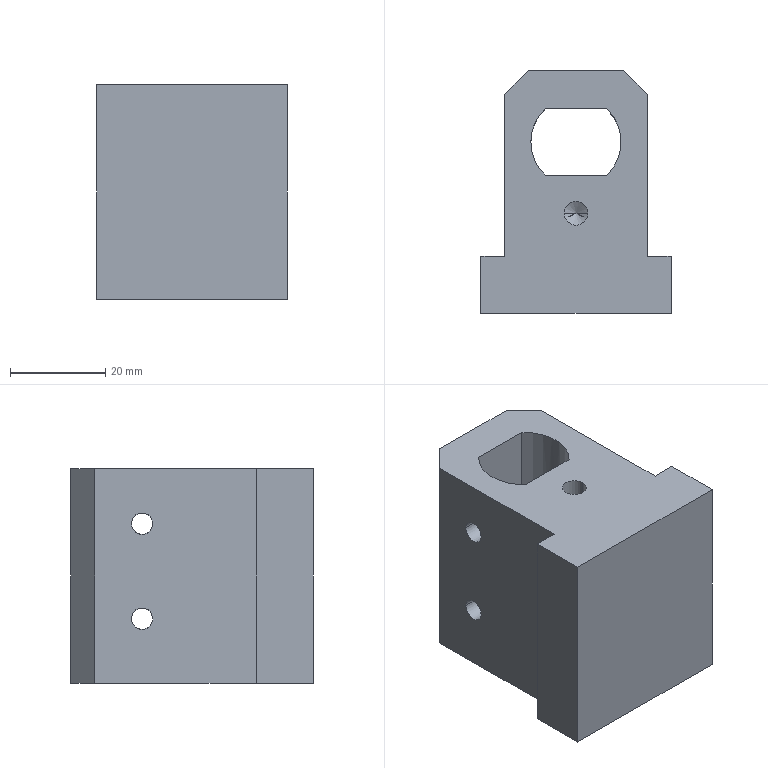Part | STEP file | magnetic tile top shaft slider | 1 solid | 37 faces | box 40 x 51 x 45 mm | volume 61253 mm3 | cylinder 17 | plane 14 | cone 6 | commonest cylinder face diameters 4.5 x8 4.2 x4 19 x3 5 x2